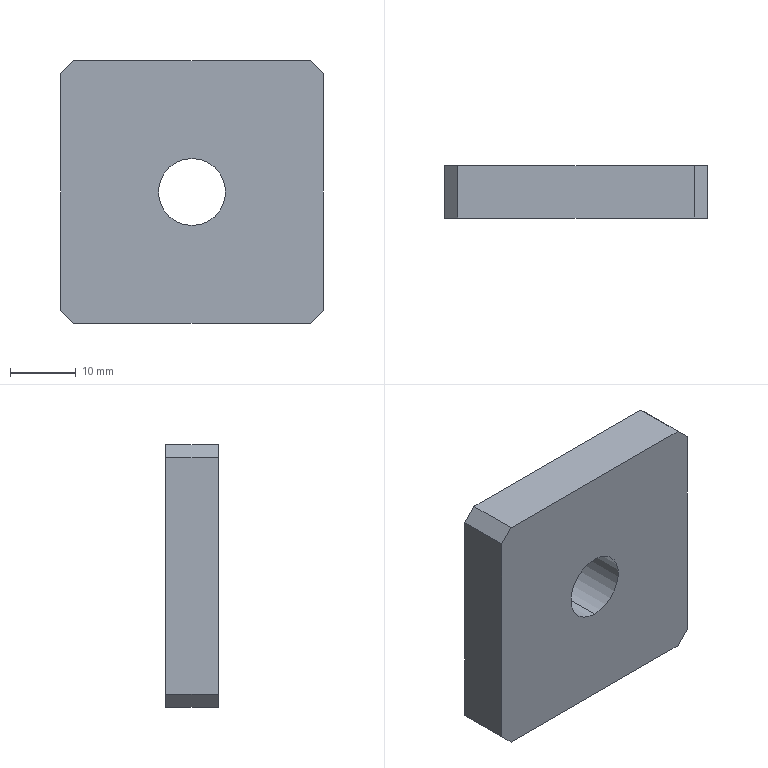Part | STEP file | Bich chan tang chinh | 1 solid | 12 faces | box 40 x 8 x 40 mm | volume 12082 mm3 | plane 10 | cylinder 2 | commonest cylinder face diameters 10.2 x2
STEP:
#1=CARTESIAN_POINT('',(0.,8.,5.1));
#2=VERTEX_POINT('',#1);
#3=CARTESIAN_POINT('',(0.,8.,-5.1));
#4=VERTEX_POINT('',#3);
#5=CARTESIAN_POINT('',(0.,8.,0.));
#6=DIRECTION('',(0.,-1.,0.));
#7=DIRECTION('',(0.,0.,-1.));
#8=AXIS2_PLACEMENT_3D('',#5,#6,#7);
#9=CIRCLE('',#8,5.1);
#10=EDGE_CURVE('',#2,#4,#9,.T.);
#11=ORIENTED_EDGE('',*,*,#10,.F.);
#12=CARTESIAN_POINT('',(0.,0.,5.1));
#13=VERTEX_POINT('',#12);
#14=CARTESIAN_POINT('',(0.,0.,5.1));
#15=DIRECTION('',(0.,-1.,0.));
#16=VECTOR('',#15,1000.);
#17=LINE('',#14,#16);
#18=EDGE_CURVE('',#2,#13,#17,.T.);
#19=ORIENTED_EDGE('',*,*,#18,.T.);
#20=CARTESIAN_POINT('',(0.,0.,-5.1));
#21=VERTEX_POINT('',#20);
#22=CARTESIAN_POINT('',(0.,0.,0.));
#23=DIRECTION('',(0.,-1.,0.));
#24=DIRECTION('',(0.,0.,-1.));
#25=AXIS2_PLACEMENT_3D('',#22,#23,#24);
#26=CIRCLE('',#25,5.1);
#27=EDGE_CURVE('',#13,#21,#26,.T.);
#28=ORIENTED_EDGE('',*,*,#27,.T.);
#29=CARTESIAN_POINT('',(0.,0.,-5.1));
#30=DIRECTION('',(0.,-1.,0.));
#31=VECTOR('',#30,1000.);
#32=LINE('',#29,#31);
#33=EDGE_CURVE('',#4,#21,#32,.T.);
#34=ORIENTED_EDGE('',*,*,#33,.F.);
#35=EDGE_LOOP('',(#11,#19,#28,#34));
#36=FACE_OUTER_BOUND('',#35,.T.);
#37=CARTESIAN_POINT('',(0.,0.,0.));
#38=DIRECTION('',(0.,-1.,0.));
#39=DIRECTION('',(0.,0.,-1.));
#40=AXIS2_PLACEMENT_3D('',#37,#38,#39);
#41=CYLINDRICAL_SURFACE('',#40,5.1);
#42=ADVANCED_FACE('',(#36),#41,.F.);
#43=CARTESIAN_POINT('',(20.,0.,18.));
#44=VERTEX_POINT('',#43);
#45=CARTESIAN_POINT('',(20.,0.,-18.));
#46=VERTEX_POINT('',#45);
#47=CARTESIAN_POINT('',(20.,0.,20.));
#48=DIRECTION('',(0.,0.,-1.));
#49=VECTOR('',#48,1000.);
#50=LINE('',#47,#49);
#51=EDGE_CURVE('',#44,#46,#50,.T.);
#52=ORIENTED_EDGE('',*,*,#51,.T.);
#53=CARTESIAN_POINT('',(20.,8.,-18.));
#54=VERTEX_POINT('',#53);
#55=CARTESIAN_POINT('',(20.,8.,-18.));
#56=DIRECTION('',(0.,1.,0.));
#57=VECTOR('',#56,1000.);
#58=LINE('',#55,#57);
#59=EDGE_CURVE('',#46,#54,#58,.T.);
#60=ORIENTED_EDGE('',*,*,#59,.T.);
#61=CARTESIAN_POINT('',(20.,8.,18.));
#62=VERTEX_POINT('',#61);
#63=CARTESIAN_POINT('',(20.,8.,20.));
#64=DIRECTION('',(0.,0.,-1.));
#65=VECTOR('',#64,1000.);
#66=LINE('',#63,#65);
#67=EDGE_CURVE('',#62,#54,#66,.T.);
#68=ORIENTED_EDGE('',*,*,#67,.F.);
#69=CARTESIAN_POINT('',(20.,8.,18.));
#70=DIRECTION('',(0.,-1.,0.));
#71=VECTOR('',#70,1000.);
#72=LINE('',#69,#71);
#73=EDGE_CURVE('',#62,#44,#72,.T.);
#74=ORIENTED_EDGE('',*,*,#73,.T.);
#75=EDGE_LOOP('',(#52,#60,#68,#74));
#76=FACE_OUTER_BOUND('',#75,.T.);
#77=CARTESIAN_POINT('',(20.,8.,20.));
#78=DIRECTION('',(-1.,0.,0.));
#79=DIRECTION('',(0.,0.,1.));
#80=AXIS2_PLACEMENT_3D('',#77,#78,#79);
#81=PLANE('',#80);
#82=ADVANCED_FACE('',(#76),#81,.F.);
#83=CARTESIAN_POINT('',(18.,0.,-20.));
#84=VERTEX_POINT('',#83);
#85=CARTESIAN_POINT('',(-18.,0.,-20.));
#86=VERTEX_POINT('',#85);
#87=CARTESIAN_POINT('',(-20.,0.,-20.));
#88=DIRECTION('',(-1.,0.,0.));
#89=VECTOR('',#88,1000.);
#90=LINE('',#87,#89);
#91=EDGE_CURVE('',#84,#86,#90,.T.);
#92=ORIENTED_EDGE('',*,*,#91,.T.);
#93=CARTESIAN_POINT('',(-18.,8.,-20.));
#94=VERTEX_POINT('',#93);
#95=CARTESIAN_POINT('',(-18.,8.,-20.));
#96=DIRECTION('',(0.,1.,0.));
#97=VECTOR('',#96,1000.);
#98=LINE('',#95,#97);
#99=EDGE_CURVE('',#86,#94,#98,.T.);
#100=ORIENTED_EDGE('',*,*,#99,.T.);
#101=CARTESIAN_POINT('',(18.,8.,-20.));
#102=VERTEX_POINT('',#101);
#103=CARTESIAN_POINT('',(-20.,8.,-20.));
#104=DIRECTION('',(-1.,0.,0.));
#105=VECTOR('',#104,1000.);
#106=LINE('',#103,#105);
#107=EDGE_CURVE('',#102,#94,#106,.T.);
#108=ORIENTED_EDGE('',*,*,#107,.F.);
#109=CARTESIAN_POINT('',(18.,8.,-20.));
#110=DIRECTION('',(0.,-1.,0.));
#111=VECTOR('',#110,1000.);
#112=LINE('',#109,#111);
#113=EDGE_CURVE('',#102,#84,#112,.T.);
#114=ORIENTED_EDGE('',*,*,#113,.T.);
#115=EDGE_LOOP('',(#92,#100,#108,#114));
#116=FACE_OUTER_BOUND('',#115,.T.);
#117=CARTESIAN_POINT('',(-20.,8.,-20.));
#118=DIRECTION('',(0.,0.,1.));
#119=DIRECTION('',(1.,0.,0.));
#120=AXIS2_PLACEMENT_3D('',#117,#118,#119);
#121=PLANE('',#120);
#122=ADVANCED_FACE('',(#116),#121,.F.);
#123=CARTESIAN_POINT('',(-20.,8.,-18.));
#124=VERTEX_POINT('',#123);
#125=CARTESIAN_POINT('',(-20.,8.,18.));
#126=VERTEX_POINT('',#125);
#127=CARTESIAN_POINT('',(-20.,8.,20.));
#128=DIRECTION('',(0.,0.,1.));
#129=VECTOR('',#128,1000.);
#130=LINE('',#127,#129);
#131=EDGE_CURVE('',#124,#126,#130,.T.);
#132=ORIENTED_EDGE('',*,*,#131,.F.);
#133=CARTESIAN_POINT('',(-20.,0.,-18.));
#134=VERTEX_POINT('',#133);
#135=CARTESIAN_POINT('',(-20.,8.,-18.));
#136=DIRECTION('',(0.,-1.,0.));
#137=VECTOR('',#136,1000.);
#138=LINE('',#135,#137);
#139=EDGE_CURVE('',#124,#134,#138,.T.);
#140=ORIENTED_EDGE('',*,*,#139,.T.);
#141=CARTESIAN_POINT('',(-20.,0.,18.));
#142=VERTEX_POINT('',#141);
#143=CARTESIAN_POINT('',(-20.,0.,20.));
#144=DIRECTION('',(0.,0.,1.));
#145=VECTOR('',#144,1000.);
#146=LINE('',#143,#145);
#147=EDGE_CURVE('',#134,#142,#146,.T.);
#148=ORIENTED_EDGE('',*,*,#147,.T.);
#149=CARTESIAN_POINT('',(-20.,8.,18.));
#150=DIRECTION('',(0.,1.,0.));
#151=VECTOR('',#150,1000.);
#152=LINE('',#149,#151);
#153=EDGE_CURVE('',#142,#126,#152,.T.);
#154=ORIENTED_EDGE('',*,*,#153,.T.);
#155=EDGE_LOOP('',(#132,#140,#148,#154));
#156=FACE_OUTER_BOUND('',#155,.T.);
#157=CARTESIAN_POINT('',(-20.,8.,20.));
#158=DIRECTION('',(1.,0.,0.));
#159=DIRECTION('',(0.,0.,-1.));
#160=AXIS2_PLACEMENT_3D('',#157,#158,#159);
#161=PLANE('',#160);
#162=ADVANCED_FACE('',(#156),#161,.F.);
#163=CARTESIAN_POINT('',(-18.,0.,20.));
#164=VERTEX_POINT('',#163);
#165=CARTESIAN_POINT('',(18.,0.,20.));
#166=VERTEX_POINT('',#165);
#167=CARTESIAN_POINT('',(-20.,0.,20.));
#168=DIRECTION('',(1.,0.,0.));
#169=VECTOR('',#168,1000.);
#170=LINE('',#167,#169);
#171=EDGE_CURVE('',#164,#166,#170,.T.);
#172=ORIENTED_EDGE('',*,*,#171,.T.);
#173=CARTESIAN_POINT('',(18.,8.,20.));
#174=VERTEX_POINT('',#173);
#175=CARTESIAN_POINT('',(18.,8.,20.));
#176=DIRECTION('',(0.,1.,0.));
#177=VECTOR('',#176,1000.);
#178=LINE('',#175,#177);
#179=EDGE_CURVE('',#166,#174,#178,.T.);
#180=ORIENTED_EDGE('',*,*,#179,.T.);
#181=CARTESIAN_POINT('',(-18.,8.,20.));
#182=VERTEX_POINT('',#181);
#183=CARTESIAN_POINT('',(-20.,8.,20.));
#184=DIRECTION('',(1.,0.,0.));
#185=VECTOR('',#184,1000.);
#186=LINE('',#183,#185);
#187=EDGE_CURVE('',#182,#174,#186,.T.);
#188=ORIENTED_EDGE('',*,*,#187,.F.);
#189=CARTESIAN_POINT('',(-18.,8.,20.));
#190=DIRECTION('',(0.,-1.,0.));
#191=VECTOR('',#190,1000.);
#192=LINE('',#189,#191);
#193=EDGE_CURVE('',#182,#164,#192,.T.);
#194=ORIENTED_EDGE('',*,*,#193,.T.);
#195=EDGE_LOOP('',(#172,#180,#188,#194));
#196=FACE_OUTER_BOUND('',#195,.T.);
#197=CARTESIAN_POINT('',(-20.,8.,20.));
#198=DIRECTION('',(0.,0.,-1.));
#199=DIRECTION('',(-1.,0.,0.));
#200=AXIS2_PLACEMENT_3D('',#197,#198,#199);
#201=PLANE('',#200);
#202=ADVANCED_FACE('',(#196),#201,.F.);
#203=CARTESIAN_POINT('',(0.,8.,0.));
#204=DIRECTION('',(0.,-1.,0.));
#205=DIRECTION('',(0.,0.,-1.));
#206=AXIS2_PLACEMENT_3D('',#203,#204,#205);
#207=CIRCLE('',#206,5.1);
#208=EDGE_CURVE('',#4,#2,#207,.T.);
#209=ORIENTED_EDGE('',*,*,#208,.T.);
#210=ORIENTED_EDGE('',*,*,#10,.T.);
#211=EDGE_LOOP('',(#209,#210));
#212=FACE_BOUND('',#211,.T.);
#213=ORIENTED_EDGE('',*,*,#107,.T.);
#214=CARTESIAN_POINT('',(-20.,8.,-18.));
#215=DIRECTION('',(-0.7071,0.,0.7071));
#216=VECTOR('',#215,1000.);
#217=LINE('',#214,#216);
#218=EDGE_CURVE('',#94,#124,#217,.T.);
#219=ORIENTED_EDGE('',*,*,#218,.T.);
#220=ORIENTED_EDGE('',*,*,#131,.T.);
#221=CARTESIAN_POINT('',(-18.,8.,20.));
#222=DIRECTION('',(0.7071,0.,0.7071));
#223=VECTOR('',#222,1000.);
#224=LINE('',#221,#223);
#225=EDGE_CURVE('',#126,#182,#224,.T.);
#226=ORIENTED_EDGE('',*,*,#225,.T.);
#227=ORIENTED_EDGE('',*,*,#187,.T.);
#228=CARTESIAN_POINT('',(20.,8.,18.));
#229=DIRECTION('',(0.7071,0.,-0.7071));
#230=VECTOR('',#229,1000.);
#231=LINE('',#228,#230);
#232=EDGE_CURVE('',#174,#62,#231,.T.);
#233=ORIENTED_EDGE('',*,*,#232,.T.);
#234=ORIENTED_EDGE('',*,*,#67,.T.);
#235=CARTESIAN_POINT('',(18.,8.,-20.));
#236=DIRECTION('',(-0.7071,0.,-0.7071));
#237=VECTOR('',#236,1000.);
#238=LINE('',#235,#237);
#239=EDGE_CURVE('',#54,#102,#238,.T.);
#240=ORIENTED_EDGE('',*,*,#239,.T.);
#241=EDGE_LOOP('',(#213,#219,#220,#226,#227,#233,#234,#240));
#242=FACE_OUTER_BOUND('',#241,.T.);
#243=CARTESIAN_POINT('',(0.,8.,0.));
#244=DIRECTION('',(0.,-1.,0.));
#245=DIRECTION('',(0.,0.,-1.));
#246=AXIS2_PLACEMENT_3D('',#243,#244,#245);
#247=PLANE('',#246);
#248=ADVANCED_FACE('',(#212,#242),#247,.F.);
#249=CARTESIAN_POINT('',(0.,0.,0.));
#250=DIRECTION('',(0.,-1.,0.));
#251=DIRECTION('',(0.,0.,-1.));
#252=AXIS2_PLACEMENT_3D('',#249,#250,#251);
#253=CIRCLE('',#252,5.1);
#254=EDGE_CURVE('',#21,#13,#253,.T.);
#255=ORIENTED_EDGE('',*,*,#254,.F.);
#256=ORIENTED_EDGE('',*,*,#27,.F.);
#257=EDGE_LOOP('',(#255,#256));
#258=FACE_BOUND('',#257,.T.);
#259=ORIENTED_EDGE('',*,*,#147,.F.);
#260=CARTESIAN_POINT('',(-19.,0.,-19.));
#261=DIRECTION('',(0.7071,0.,-0.7071));
#262=VECTOR('',#261,1000.);
#263=LINE('',#260,#262);
#264=EDGE_CURVE('',#134,#86,#263,.T.);
#265=ORIENTED_EDGE('',*,*,#264,.T.);
#266=ORIENTED_EDGE('',*,*,#91,.F.);
#267=CARTESIAN_POINT('',(19.,0.,-19.));
#268=DIRECTION('',(0.7071,0.,0.7071));
#269=VECTOR('',#268,1000.);
#270=LINE('',#267,#269);
#271=EDGE_CURVE('',#84,#46,#270,.T.);
#272=ORIENTED_EDGE('',*,*,#271,.T.);
#273=ORIENTED_EDGE('',*,*,#51,.F.);
#274=CARTESIAN_POINT('',(19.,0.,19.));
#275=DIRECTION('',(-0.7071,0.,0.7071));
#276=VECTOR('',#275,1000.);
#277=LINE('',#274,#276);
#278=EDGE_CURVE('',#44,#166,#277,.T.);
#279=ORIENTED_EDGE('',*,*,#278,.T.);
#280=ORIENTED_EDGE('',*,*,#171,.F.);
#281=CARTESIAN_POINT('',(-19.,0.,19.));
#282=DIRECTION('',(-0.7071,0.,-0.7071));
#283=VECTOR('',#282,1000.);
#284=LINE('',#281,#283);
#285=EDGE_CURVE('',#164,#142,#284,.T.);
#286=ORIENTED_EDGE('',*,*,#285,.T.);
#287=EDGE_LOOP('',(#259,#265,#266,#272,#273,#279,#280,#286));
#288=FACE_OUTER_BOUND('',#287,.T.);
#289=CARTESIAN_POINT('',(0.,0.,0.));
#290=DIRECTION('',(0.,-1.,0.));
#291=DIRECTION('',(0.,0.,-1.));
#292=AXIS2_PLACEMENT_3D('',#289,#290,#291);
#293=PLANE('',#292);
#294=ADVANCED_FACE('',(#258,#288),#293,.T.);
#295=ORIENTED_EDGE('',*,*,#218,.F.);
#296=ORIENTED_EDGE('',*,*,#99,.F.);
#297=ORIENTED_EDGE('',*,*,#264,.F.);
#298=ORIENTED_EDGE('',*,*,#139,.F.);
#299=EDGE_LOOP('',(#295,#296,#297,#298));
#300=FACE_OUTER_BOUND('',#299,.T.);
#301=CARTESIAN_POINT('',(-20.,8.,-18.));
#302=DIRECTION('',(0.7071,0.,0.7071));
#303=DIRECTION('',(0.,-1.,0.));
#304=AXIS2_PLACEMENT_3D('',#301,#302,#303);
#305=PLANE('',#304);
#306=ADVANCED_FACE('',(#300),#305,.F.);
#307=ORIENTED_EDGE('',*,*,#239,.F.);
#308=ORIENTED_EDGE('',*,*,#59,.F.);
#309=ORIENTED_EDGE('',*,*,#271,.F.);
#310=ORIENTED_EDGE('',*,*,#113,.F.);
#311=EDGE_LOOP('',(#307,#308,#309,#310));
#312=FACE_OUTER_BOUND('',#311,.T.);
#313=CARTESIAN_POINT('',(18.,8.,-20.));
#314=DIRECTION('',(-0.7071,0.,0.7071));
#315=DIRECTION('',(0.,-1.,0.));
#316=AXIS2_PLACEMENT_3D('',#313,#314,#315);
#317=PLANE('',#316);
#318=ADVANCED_FACE('',(#312),#317,.F.);
#319=ORIENTED_EDGE('',*,*,#232,.F.);
#320=ORIENTED_EDGE('',*,*,#179,.F.);
#321=ORIENTED_EDGE('',*,*,#278,.F.);
#322=ORIENTED_EDGE('',*,*,#73,.F.);
#323=EDGE_LOOP('',(#319,#320,#321,#322));
#324=FACE_OUTER_BOUND('',#323,.T.);
#325=CARTESIAN_POINT('',(20.,8.,18.));
#326=DIRECTION('',(-0.7071,0.,-0.7071));
#327=DIRECTION('',(0.,-1.,0.));
#328=AXIS2_PLACEMENT_3D('',#325,#326,#327);
#329=PLANE('',#328);
#330=ADVANCED_FACE('',(#324),#329,.F.);
#331=ORIENTED_EDGE('',*,*,#225,.F.);
#332=ORIENTED_EDGE('',*,*,#153,.F.);
#333=ORIENTED_EDGE('',*,*,#285,.F.);
#334=ORIENTED_EDGE('',*,*,#193,.F.);
#335=EDGE_LOOP('',(#331,#332,#333,#334));
#336=FACE_OUTER_BOUND('',#335,.T.);
#337=CARTESIAN_POINT('',(-18.,8.,20.));
#338=DIRECTION('',(0.7071,0.,-0.7071));
#339=DIRECTION('',(0.,-1.,0.));
#340=AXIS2_PLACEMENT_3D('',#337,#338,#339);
#341=PLANE('',#340);
#342=ADVANCED_FACE('',(#336),#341,.F.);
#343=ORIENTED_EDGE('',*,*,#18,.F.);
#344=ORIENTED_EDGE('',*,*,#208,.F.);
#345=ORIENTED_EDGE('',*,*,#33,.T.);
#346=ORIENTED_EDGE('',*,*,#254,.T.);
#347=EDGE_LOOP('',(#343,#344,#345,#346));
#348=FACE_OUTER_BOUND('',#347,.T.);
#349=CARTESIAN_POINT('',(0.,0.,0.));
#350=DIRECTION('',(0.,-1.,0.));
#351=DIRECTION('',(0.,0.,-1.));
#352=AXIS2_PLACEMENT_3D('',#349,#350,#351);
#353=CYLINDRICAL_SURFACE('',#352,5.1);
#354=ADVANCED_FACE('',(#348),#353,.F.);
#355=CLOSED_SHELL('',(#42,#82,#122,#162,#202,#248,#294,#306,#318,#330,#342,#354));
#356=MANIFOLD_SOLID_BREP('',#355);
#357=CARTESIAN_POINT('',(0.,0.,0.));
#358=DIRECTION('',(0.,0.,1.));
#359=DIRECTION('',(1.,0.,0.));
#360=AXIS2_PLACEMENT_3D('',#357,#358,#359);
#361=(LENGTH_UNIT()NAMED_UNIT(*)SI_UNIT(.MILLI.,.METRE.));
#362=UNCERTAINTY_MEASURE_WITH_UNIT(LENGTH_MEASURE(0.00001),#361,'','');
#363=(NAMED_UNIT(*)PLANE_ANGLE_UNIT()SI_UNIT($,.RADIAN.));
#364=(NAMED_UNIT(*)SI_UNIT($,.STERADIAN.)SOLID_ANGLE_UNIT());
#365=(GEOMETRIC_REPRESENTATION_CONTEXT(3)GLOBAL_UNCERTAINTY_ASSIGNED_CONTEXT((#362))GLOBAL_UNIT_ASSIGNED_CONTEXT((#361,#363,#364))REPRESENTATION_CONTEXT('',''));
#366=ADVANCED_BREP_SHAPE_REPRESENTATION('',(#356,#360),#365);